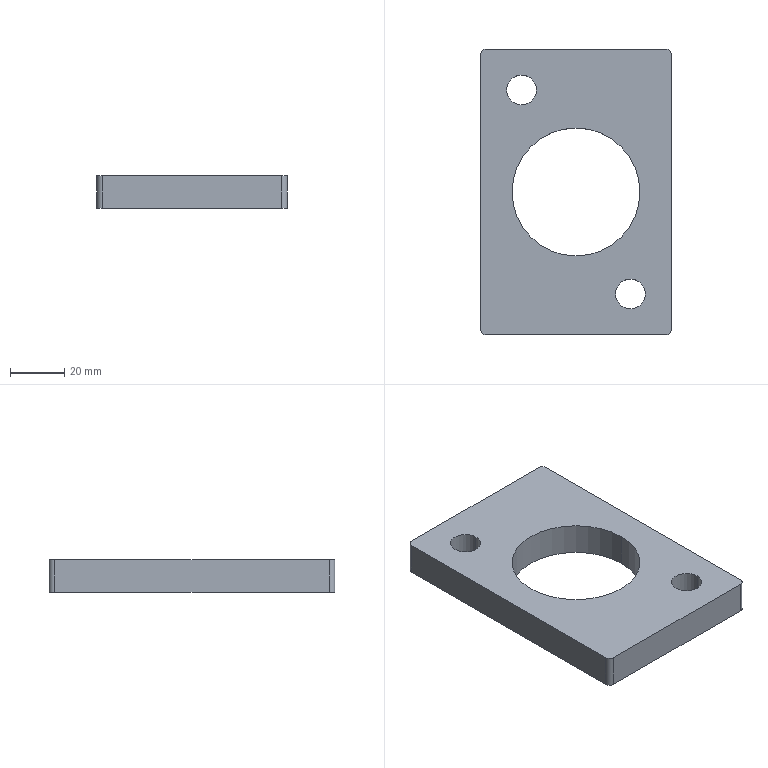Part | SolidWorks | features Extrusion 1 | 1 solid | 16 faces | box 70 x 105 x 12 mm | volume 65059 mm3 | cylinder 10 | plane 6 | commonest cylinder face diameters 4 x4 11 x4 47 x2
STEP:
#1=CARTESIAN_POINT('',(14.5,-37.5,12.));
#2=VERTEX_POINT('',#1);
#3=CARTESIAN_POINT('',(25.5,-37.5,12.));
#4=VERTEX_POINT('',#3);
#5=CARTESIAN_POINT('',(20.,-37.5,12.));
#6=DIRECTION('',(0.,0.,1.));
#7=DIRECTION('',(1.,0.,0.));
#8=AXIS2_PLACEMENT_3D('',#5,#6,#7);
#9=CIRCLE('',#8,5.5);
#10=EDGE_CURVE('',#2,#4,#9,.T.);
#11=ORIENTED_EDGE('',*,*,#10,.T.);
#12=CARTESIAN_POINT('',(25.5,-37.5,0.));
#13=VERTEX_POINT('',#12);
#14=CARTESIAN_POINT('',(25.5,-37.5,12.));
#15=DIRECTION('',(0.,0.,-1.));
#16=VECTOR('',#15,1000.);
#17=LINE('',#14,#16);
#18=EDGE_CURVE('',#4,#13,#17,.T.);
#19=ORIENTED_EDGE('',*,*,#18,.T.);
#20=CARTESIAN_POINT('',(14.5,-37.5,0.));
#21=VERTEX_POINT('',#20);
#22=CARTESIAN_POINT('',(20.,-37.5,0.));
#23=DIRECTION('',(0.,0.,1.));
#24=DIRECTION('',(1.,0.,0.));
#25=AXIS2_PLACEMENT_3D('',#22,#23,#24);
#26=CIRCLE('',#25,5.5);
#27=EDGE_CURVE('',#21,#13,#26,.T.);
#28=ORIENTED_EDGE('',*,*,#27,.F.);
#29=CARTESIAN_POINT('',(14.5,-37.5,12.));
#30=DIRECTION('',(0.,0.,-1.));
#31=VECTOR('',#30,1000.);
#32=LINE('',#29,#31);
#33=EDGE_CURVE('',#2,#21,#32,.T.);
#34=ORIENTED_EDGE('',*,*,#33,.F.);
#35=EDGE_LOOP('',(#11,#19,#28,#34));
#36=FACE_OUTER_BOUND('',#35,.T.);
#37=CARTESIAN_POINT('',(20.,-37.5,12.));
#38=DIRECTION('',(0.,0.,-1.));
#39=DIRECTION('',(-1.,0.,0.));
#40=AXIS2_PLACEMENT_3D('',#37,#38,#39);
#41=CYLINDRICAL_SURFACE('',#40,5.5);
#42=ADVANCED_FACE('',(#36),#41,.F.);
#43=CARTESIAN_POINT('',(-25.5,37.5,12.));
#44=VERTEX_POINT('',#43);
#45=CARTESIAN_POINT('',(-14.5,37.5,12.));
#46=VERTEX_POINT('',#45);
#47=CARTESIAN_POINT('',(-20.,37.5,12.));
#48=DIRECTION('',(0.,0.,1.));
#49=DIRECTION('',(1.,0.,0.));
#50=AXIS2_PLACEMENT_3D('',#47,#48,#49);
#51=CIRCLE('',#50,5.5);
#52=EDGE_CURVE('',#44,#46,#51,.T.);
#53=ORIENTED_EDGE('',*,*,#52,.T.);
#54=CARTESIAN_POINT('',(-14.5,37.5,0.));
#55=VERTEX_POINT('',#54);
#56=CARTESIAN_POINT('',(-14.5,37.5,12.));
#57=DIRECTION('',(0.,0.,-1.));
#58=VECTOR('',#57,1000.);
#59=LINE('',#56,#58);
#60=EDGE_CURVE('',#46,#55,#59,.T.);
#61=ORIENTED_EDGE('',*,*,#60,.T.);
#62=CARTESIAN_POINT('',(-25.5,37.5,0.));
#63=VERTEX_POINT('',#62);
#64=CARTESIAN_POINT('',(-20.,37.5,0.));
#65=DIRECTION('',(0.,0.,1.));
#66=DIRECTION('',(1.,0.,0.));
#67=AXIS2_PLACEMENT_3D('',#64,#65,#66);
#68=CIRCLE('',#67,5.5);
#69=EDGE_CURVE('',#63,#55,#68,.T.);
#70=ORIENTED_EDGE('',*,*,#69,.F.);
#71=CARTESIAN_POINT('',(-25.5,37.5,12.));
#72=DIRECTION('',(0.,0.,-1.));
#73=VECTOR('',#72,1000.);
#74=LINE('',#71,#73);
#75=EDGE_CURVE('',#44,#63,#74,.T.);
#76=ORIENTED_EDGE('',*,*,#75,.F.);
#77=EDGE_LOOP('',(#53,#61,#70,#76));
#78=FACE_OUTER_BOUND('',#77,.T.);
#79=CARTESIAN_POINT('',(-20.,37.5,12.));
#80=DIRECTION('',(0.,0.,-1.));
#81=DIRECTION('',(-1.,0.,0.));
#82=AXIS2_PLACEMENT_3D('',#79,#80,#81);
#83=CYLINDRICAL_SURFACE('',#82,5.5);
#84=ADVANCED_FACE('',(#78),#83,.F.);
#85=CARTESIAN_POINT('',(-23.5,0.,12.));
#86=VERTEX_POINT('',#85);
#87=CARTESIAN_POINT('',(23.5,0.,12.));
#88=VERTEX_POINT('',#87);
#89=CARTESIAN_POINT('',(0.,0.,12.));
#90=DIRECTION('',(0.,0.,1.));
#91=DIRECTION('',(1.,0.,0.));
#92=AXIS2_PLACEMENT_3D('',#89,#90,#91);
#93=CIRCLE('',#92,23.5);
#94=EDGE_CURVE('',#86,#88,#93,.T.);
#95=ORIENTED_EDGE('',*,*,#94,.T.);
#96=CARTESIAN_POINT('',(23.5,0.,0.));
#97=VERTEX_POINT('',#96);
#98=CARTESIAN_POINT('',(23.5,0.,12.));
#99=DIRECTION('',(0.,0.,-1.));
#100=VECTOR('',#99,1000.);
#101=LINE('',#98,#100);
#102=EDGE_CURVE('',#88,#97,#101,.T.);
#103=ORIENTED_EDGE('',*,*,#102,.T.);
#104=CARTESIAN_POINT('',(-23.5,0.,0.));
#105=VERTEX_POINT('',#104);
#106=CARTESIAN_POINT('',(0.,0.,0.));
#107=DIRECTION('',(0.,0.,1.));
#108=DIRECTION('',(1.,0.,0.));
#109=AXIS2_PLACEMENT_3D('',#106,#107,#108);
#110=CIRCLE('',#109,23.5);
#111=EDGE_CURVE('',#105,#97,#110,.T.);
#112=ORIENTED_EDGE('',*,*,#111,.F.);
#113=CARTESIAN_POINT('',(-23.5,0.,12.));
#114=DIRECTION('',(0.,0.,-1.));
#115=VECTOR('',#114,1000.);
#116=LINE('',#113,#115);
#117=EDGE_CURVE('',#86,#105,#116,.T.);
#118=ORIENTED_EDGE('',*,*,#117,.F.);
#119=EDGE_LOOP('',(#95,#103,#112,#118));
#120=FACE_OUTER_BOUND('',#119,.T.);
#121=CARTESIAN_POINT('',(0.,0.,12.));
#122=DIRECTION('',(0.,0.,-1.));
#123=DIRECTION('',(-1.,0.,0.));
#124=AXIS2_PLACEMENT_3D('',#121,#122,#123);
#125=CYLINDRICAL_SURFACE('',#124,23.5);
#126=ADVANCED_FACE('',(#120),#125,.F.);
#127=ORIENTED_EDGE('',*,*,#52,.F.);
#128=CARTESIAN_POINT('',(-20.,37.5,12.));
#129=DIRECTION('',(0.,0.,1.));
#130=DIRECTION('',(1.,0.,0.));
#131=AXIS2_PLACEMENT_3D('',#128,#129,#130);
#132=CIRCLE('',#131,5.5);
#133=EDGE_CURVE('',#46,#44,#132,.T.);
#134=ORIENTED_EDGE('',*,*,#133,.F.);
#135=EDGE_LOOP('',(#127,#134));
#136=FACE_BOUND('',#135,.T.);
#137=CARTESIAN_POINT('',(-33.,52.5,12.));
#138=VERTEX_POINT('',#137);
#139=CARTESIAN_POINT('',(-35.,50.5,12.));
#140=VERTEX_POINT('',#139);
#141=CARTESIAN_POINT('',(-33.,50.5,12.));
#142=DIRECTION('',(0.,0.,1.));
#143=DIRECTION('',(1.,0.,0.));
#144=AXIS2_PLACEMENT_3D('',#141,#142,#143);
#145=CIRCLE('',#144,2.);
#146=EDGE_CURVE('',#138,#140,#145,.T.);
#147=ORIENTED_EDGE('',*,*,#146,.T.);
#148=CARTESIAN_POINT('',(-35.,-50.5,12.));
#149=VERTEX_POINT('',#148);
#150=CARTESIAN_POINT('',(-35.,50.5,12.));
#151=DIRECTION('',(0.,-1.,0.));
#152=VECTOR('',#151,1000.);
#153=LINE('',#150,#152);
#154=EDGE_CURVE('',#140,#149,#153,.T.);
#155=ORIENTED_EDGE('',*,*,#154,.T.);
#156=CARTESIAN_POINT('',(-33.,-52.5,12.));
#157=VERTEX_POINT('',#156);
#158=CARTESIAN_POINT('',(-33.,-50.5,12.));
#159=DIRECTION('',(0.,0.,1.));
#160=DIRECTION('',(1.,0.,0.));
#161=AXIS2_PLACEMENT_3D('',#158,#159,#160);
#162=CIRCLE('',#161,2.);
#163=EDGE_CURVE('',#149,#157,#162,.T.);
#164=ORIENTED_EDGE('',*,*,#163,.T.);
#165=CARTESIAN_POINT('',(33.,-52.5,12.));
#166=VERTEX_POINT('',#165);
#167=CARTESIAN_POINT('',(-33.,-52.5,12.));
#168=DIRECTION('',(1.,0.,0.));
#169=VECTOR('',#168,1000.);
#170=LINE('',#167,#169);
#171=EDGE_CURVE('',#157,#166,#170,.T.);
#172=ORIENTED_EDGE('',*,*,#171,.T.);
#173=CARTESIAN_POINT('',(35.,-50.5,12.));
#174=VERTEX_POINT('',#173);
#175=CARTESIAN_POINT('',(33.,-50.5,12.));
#176=DIRECTION('',(0.,0.,1.));
#177=DIRECTION('',(1.,0.,0.));
#178=AXIS2_PLACEMENT_3D('',#175,#176,#177);
#179=CIRCLE('',#178,2.);
#180=EDGE_CURVE('',#166,#174,#179,.T.);
#181=ORIENTED_EDGE('',*,*,#180,.T.);
#182=CARTESIAN_POINT('',(35.,50.5,12.));
#183=VERTEX_POINT('',#182);
#184=CARTESIAN_POINT('',(35.,50.5,12.));
#185=DIRECTION('',(0.,1.,0.));
#186=VECTOR('',#185,1000.);
#187=LINE('',#184,#186);
#188=EDGE_CURVE('',#174,#183,#187,.T.);
#189=ORIENTED_EDGE('',*,*,#188,.T.);
#190=CARTESIAN_POINT('',(33.,52.5,12.));
#191=VERTEX_POINT('',#190);
#192=CARTESIAN_POINT('',(33.,50.5,12.));
#193=DIRECTION('',(0.,0.,1.));
#194=DIRECTION('',(-1.,0.,0.));
#195=AXIS2_PLACEMENT_3D('',#192,#193,#194);
#196=CIRCLE('',#195,2.);
#197=EDGE_CURVE('',#183,#191,#196,.T.);
#198=ORIENTED_EDGE('',*,*,#197,.T.);
#199=CARTESIAN_POINT('',(-33.,52.5,12.));
#200=DIRECTION('',(-1.,0.,0.));
#201=VECTOR('',#200,1000.);
#202=LINE('',#199,#201);
#203=EDGE_CURVE('',#191,#138,#202,.T.);
#204=ORIENTED_EDGE('',*,*,#203,.T.);
#205=EDGE_LOOP('',(#147,#155,#164,#172,#181,#189,#198,#204));
#206=FACE_OUTER_BOUND('',#205,.T.);
#207=ORIENTED_EDGE('',*,*,#94,.F.);
#208=CARTESIAN_POINT('',(0.,0.,12.));
#209=DIRECTION('',(0.,0.,1.));
#210=DIRECTION('',(1.,0.,0.));
#211=AXIS2_PLACEMENT_3D('',#208,#209,#210);
#212=CIRCLE('',#211,23.5);
#213=EDGE_CURVE('',#88,#86,#212,.T.);
#214=ORIENTED_EDGE('',*,*,#213,.F.);
#215=EDGE_LOOP('',(#207,#214));
#216=FACE_BOUND('',#215,.T.);
#217=ORIENTED_EDGE('',*,*,#10,.F.);
#218=CARTESIAN_POINT('',(20.,-37.5,12.));
#219=DIRECTION('',(0.,0.,1.));
#220=DIRECTION('',(1.,0.,0.));
#221=AXIS2_PLACEMENT_3D('',#218,#219,#220);
#222=CIRCLE('',#221,5.5);
#223=EDGE_CURVE('',#4,#2,#222,.T.);
#224=ORIENTED_EDGE('',*,*,#223,.F.);
#225=EDGE_LOOP('',(#217,#224));
#226=FACE_BOUND('',#225,.T.);
#227=CARTESIAN_POINT('',(-33.,50.5,12.));
#228=DIRECTION('',(0.,0.,1.));
#229=DIRECTION('',(1.,0.,0.));
#230=AXIS2_PLACEMENT_3D('',#227,#228,#229);
#231=PLANE('',#230);
#232=ADVANCED_FACE('',(#136,#206,#216,#226),#231,.T.);
#233=CARTESIAN_POINT('',(-33.,52.5,0.));
#234=VERTEX_POINT('',#233);
#235=CARTESIAN_POINT('',(-35.,50.5,0.));
#236=VERTEX_POINT('',#235);
#237=CARTESIAN_POINT('',(-33.,50.5,0.));
#238=DIRECTION('',(0.,0.,1.));
#239=DIRECTION('',(1.,0.,0.));
#240=AXIS2_PLACEMENT_3D('',#237,#238,#239);
#241=CIRCLE('',#240,2.);
#242=EDGE_CURVE('',#234,#236,#241,.T.);
#243=ORIENTED_EDGE('',*,*,#242,.F.);
#244=CARTESIAN_POINT('',(33.,52.5,0.));
#245=VERTEX_POINT('',#244);
#246=CARTESIAN_POINT('',(-33.,52.5,0.));
#247=DIRECTION('',(-1.,0.,0.));
#248=VECTOR('',#247,1000.);
#249=LINE('',#246,#248);
#250=EDGE_CURVE('',#245,#234,#249,.T.);
#251=ORIENTED_EDGE('',*,*,#250,.F.);
#252=CARTESIAN_POINT('',(35.,50.5,0.));
#253=VERTEX_POINT('',#252);
#254=CARTESIAN_POINT('',(33.,50.5,0.));
#255=DIRECTION('',(0.,0.,1.));
#256=DIRECTION('',(-1.,0.,0.));
#257=AXIS2_PLACEMENT_3D('',#254,#255,#256);
#258=CIRCLE('',#257,2.);
#259=EDGE_CURVE('',#253,#245,#258,.T.);
#260=ORIENTED_EDGE('',*,*,#259,.F.);
#261=CARTESIAN_POINT('',(35.,-50.5,0.));
#262=VERTEX_POINT('',#261);
#263=CARTESIAN_POINT('',(35.,50.5,0.));
#264=DIRECTION('',(0.,1.,0.));
#265=VECTOR('',#264,1000.);
#266=LINE('',#263,#265);
#267=EDGE_CURVE('',#262,#253,#266,.T.);
#268=ORIENTED_EDGE('',*,*,#267,.F.);
#269=CARTESIAN_POINT('',(33.,-52.5,0.));
#270=VERTEX_POINT('',#269);
#271=CARTESIAN_POINT('',(33.,-50.5,0.));
#272=DIRECTION('',(0.,0.,1.));
#273=DIRECTION('',(1.,0.,0.));
#274=AXIS2_PLACEMENT_3D('',#271,#272,#273);
#275=CIRCLE('',#274,2.);
#276=EDGE_CURVE('',#270,#262,#275,.T.);
#277=ORIENTED_EDGE('',*,*,#276,.F.);
#278=CARTESIAN_POINT('',(-33.,-52.5,0.));
#279=VERTEX_POINT('',#278);
#280=CARTESIAN_POINT('',(-33.,-52.5,0.));
#281=DIRECTION('',(1.,0.,0.));
#282=VECTOR('',#281,1000.);
#283=LINE('',#280,#282);
#284=EDGE_CURVE('',#279,#270,#283,.T.);
#285=ORIENTED_EDGE('',*,*,#284,.F.);
#286=CARTESIAN_POINT('',(-35.,-50.5,0.));
#287=VERTEX_POINT('',#286);
#288=CARTESIAN_POINT('',(-33.,-50.5,0.));
#289=DIRECTION('',(0.,0.,1.));
#290=DIRECTION('',(1.,0.,0.));
#291=AXIS2_PLACEMENT_3D('',#288,#289,#290);
#292=CIRCLE('',#291,2.);
#293=EDGE_CURVE('',#287,#279,#292,.T.);
#294=ORIENTED_EDGE('',*,*,#293,.F.);
#295=CARTESIAN_POINT('',(-35.,50.5,0.));
#296=DIRECTION('',(0.,-1.,0.));
#297=VECTOR('',#296,1000.);
#298=LINE('',#295,#297);
#299=EDGE_CURVE('',#236,#287,#298,.T.);
#300=ORIENTED_EDGE('',*,*,#299,.F.);
#301=EDGE_LOOP('',(#243,#251,#260,#268,#277,#285,#294,#300));
#302=FACE_OUTER_BOUND('',#301,.T.);
#303=ORIENTED_EDGE('',*,*,#111,.T.);
#304=CARTESIAN_POINT('',(0.,0.,0.));
#305=DIRECTION('',(0.,0.,1.));
#306=DIRECTION('',(1.,0.,0.));
#307=AXIS2_PLACEMENT_3D('',#304,#305,#306);
#308=CIRCLE('',#307,23.5);
#309=EDGE_CURVE('',#97,#105,#308,.T.);
#310=ORIENTED_EDGE('',*,*,#309,.T.);
#311=EDGE_LOOP('',(#303,#310));
#312=FACE_BOUND('',#311,.T.);
#313=ORIENTED_EDGE('',*,*,#69,.T.);
#314=CARTESIAN_POINT('',(-20.,37.5,0.));
#315=DIRECTION('',(0.,0.,1.));
#316=DIRECTION('',(1.,0.,0.));
#317=AXIS2_PLACEMENT_3D('',#314,#315,#316);
#318=CIRCLE('',#317,5.5);
#319=EDGE_CURVE('',#55,#63,#318,.T.);
#320=ORIENTED_EDGE('',*,*,#319,.T.);
#321=EDGE_LOOP('',(#313,#320));
#322=FACE_BOUND('',#321,.T.);
#323=ORIENTED_EDGE('',*,*,#27,.T.);
#324=CARTESIAN_POINT('',(20.,-37.5,0.));
#325=DIRECTION('',(0.,0.,1.));
#326=DIRECTION('',(1.,0.,0.));
#327=AXIS2_PLACEMENT_3D('',#324,#325,#326);
#328=CIRCLE('',#327,5.5);
#329=EDGE_CURVE('',#13,#21,#328,.T.);
#330=ORIENTED_EDGE('',*,*,#329,.T.);
#331=EDGE_LOOP('',(#323,#330));
#332=FACE_BOUND('',#331,.T.);
#333=CARTESIAN_POINT('',(-33.,50.5,0.));
#334=DIRECTION('',(0.,0.,1.));
#335=DIRECTION('',(1.,0.,0.));
#336=AXIS2_PLACEMENT_3D('',#333,#334,#335);
#337=PLANE('',#336);
#338=ADVANCED_FACE('',(#302,#312,#322,#332),#337,.F.);
#339=ORIENTED_EDGE('',*,*,#242,.T.);
#340=CARTESIAN_POINT('',(-35.,50.5,12.));
#341=DIRECTION('',(0.,0.,-1.));
#342=VECTOR('',#341,1000.);
#343=LINE('',#340,#342);
#344=EDGE_CURVE('',#140,#236,#343,.T.);
#345=ORIENTED_EDGE('',*,*,#344,.F.);
#346=ORIENTED_EDGE('',*,*,#146,.F.);
#347=CARTESIAN_POINT('',(-33.,52.5,12.));
#348=DIRECTION('',(0.,0.,-1.));
#349=VECTOR('',#348,1000.);
#350=LINE('',#347,#349);
#351=EDGE_CURVE('',#138,#234,#350,.T.);
#352=ORIENTED_EDGE('',*,*,#351,.T.);
#353=EDGE_LOOP('',(#339,#345,#346,#352));
#354=FACE_OUTER_BOUND('',#353,.T.);
#355=CARTESIAN_POINT('',(-33.,50.5,12.));
#356=DIRECTION('',(0.,0.,-1.));
#357=DIRECTION('',(-1.,0.,0.));
#358=AXIS2_PLACEMENT_3D('',#355,#356,#357);
#359=CYLINDRICAL_SURFACE('',#358,2.);
#360=ADVANCED_FACE('',(#354),#359,.T.);
#361=ORIENTED_EDGE('',*,*,#299,.T.);
#362=CARTESIAN_POINT('',(-35.,-50.5,12.));
#363=DIRECTION('',(0.,0.,-1.));
#364=VECTOR('',#363,1000.);
#365=LINE('',#362,#364);
#366=EDGE_CURVE('',#149,#287,#365,.T.);
#367=ORIENTED_EDGE('',*,*,#366,.F.);
#368=ORIENTED_EDGE('',*,*,#154,.F.);
#369=ORIENTED_EDGE('',*,*,#344,.T.);
#370=EDGE_LOOP('',(#361,#367,#368,#369));
#371=FACE_OUTER_BOUND('',#370,.T.);
#372=CARTESIAN_POINT('',(-35.,50.5,12.));
#373=DIRECTION('',(1.,0.,0.));
#374=DIRECTION('',(0.,1.,0.));
#375=AXIS2_PLACEMENT_3D('',#372,#373,#374);
#376=PLANE('',#375);
#377=ADVANCED_FACE('',(#371),#376,.F.);
#378=ORIENTED_EDGE('',*,*,#293,.T.);
#379=CARTESIAN_POINT('',(-33.,-52.5,12.));
#380=DIRECTION('',(0.,0.,-1.));
#381=VECTOR('',#380,1000.);
#382=LINE('',#379,#381);
#383=EDGE_CURVE('',#157,#279,#382,.T.);
#384=ORIENTED_EDGE('',*,*,#383,.F.);
#385=ORIENTED_EDGE('',*,*,#163,.F.);
#386=ORIENTED_EDGE('',*,*,#366,.T.);
#387=EDGE_LOOP('',(#378,#384,#385,#386));
#388=FACE_OUTER_BOUND('',#387,.T.);
#389=CARTESIAN_POINT('',(-33.,-50.5,12.));
#390=DIRECTION('',(0.,0.,-1.));
#391=DIRECTION('',(-1.,0.,0.));
#392=AXIS2_PLACEMENT_3D('',#389,#390,#391);
#393=CYLINDRICAL_SURFACE('',#392,2.);
#394=ADVANCED_FACE('',(#388),#393,.T.);
#395=ORIENTED_EDGE('',*,*,#284,.T.);
#396=CARTESIAN_POINT('',(33.,-52.5,12.));
#397=DIRECTION('',(0.,0.,-1.));
#398=VECTOR('',#397,1000.);
#399=LINE('',#396,#398);
#400=EDGE_CURVE('',#166,#270,#399,.T.);
#401=ORIENTED_EDGE('',*,*,#400,.F.);
#402=ORIENTED_EDGE('',*,*,#171,.F.);
#403=ORIENTED_EDGE('',*,*,#383,.T.);
#404=EDGE_LOOP('',(#395,#401,#402,#403));
#405=FACE_OUTER_BOUND('',#404,.T.);
#406=CARTESIAN_POINT('',(-33.,-52.5,12.));
#407=DIRECTION('',(0.,1.,0.));
#408=DIRECTION('',(0.,0.,1.));
#409=AXIS2_PLACEMENT_3D('',#406,#407,#408);
#410=PLANE('',#409);
#411=ADVANCED_FACE('',(#405),#410,.F.);
#412=ORIENTED_EDGE('',*,*,#276,.T.);
#413=CARTESIAN_POINT('',(35.,-50.5,12.));
#414=DIRECTION('',(0.,0.,-1.));
#415=VECTOR('',#414,1000.);
#416=LINE('',#413,#415);
#417=EDGE_CURVE('',#174,#262,#416,.T.);
#418=ORIENTED_EDGE('',*,*,#417,.F.);
#419=ORIENTED_EDGE('',*,*,#180,.F.);
#420=ORIENTED_EDGE('',*,*,#400,.T.);
#421=EDGE_LOOP('',(#412,#418,#419,#420));
#422=FACE_OUTER_BOUND('',#421,.T.);
#423=CARTESIAN_POINT('',(33.,-50.5,12.));
#424=DIRECTION('',(0.,0.,-1.));
#425=DIRECTION('',(-1.,0.,0.));
#426=AXIS2_PLACEMENT_3D('',#423,#424,#425);
#427=CYLINDRICAL_SURFACE('',#426,2.);
#428=ADVANCED_FACE('',(#422),#427,.T.);
#429=ORIENTED_EDGE('',*,*,#267,.T.);
#430=CARTESIAN_POINT('',(35.,50.5,12.));
#431=DIRECTION('',(0.,0.,-1.));
#432=VECTOR('',#431,1000.);
#433=LINE('',#430,#432);
#434=EDGE_CURVE('',#183,#253,#433,.T.);
#435=ORIENTED_EDGE('',*,*,#434,.F.);
#436=ORIENTED_EDGE('',*,*,#188,.F.);
#437=ORIENTED_EDGE('',*,*,#417,.T.);
#438=EDGE_LOOP('',(#429,#435,#436,#437));
#439=FACE_OUTER_BOUND('',#438,.T.);
#440=CARTESIAN_POINT('',(35.,50.5,12.));
#441=DIRECTION('',(-1.,0.,0.));
#442=DIRECTION('',(0.,-1.,0.));
#443=AXIS2_PLACEMENT_3D('',#440,#441,#442);
#444=PLANE('',#443);
#445=ADVANCED_FACE('',(#439),#444,.F.);
#446=ORIENTED_EDGE('',*,*,#259,.T.);
#447=CARTESIAN_POINT('',(33.,52.5,12.));
#448=DIRECTION('',(0.,0.,-1.));
#449=VECTOR('',#448,1000.);
#450=LINE('',#447,#449);
#451=EDGE_CURVE('',#191,#245,#450,.T.);
#452=ORIENTED_EDGE('',*,*,#451,.F.);
#453=ORIENTED_EDGE('',*,*,#197,.F.);
#454=ORIENTED_EDGE('',*,*,#434,.T.);
#455=EDGE_LOOP('',(#446,#452,#453,#454));
#456=FACE_OUTER_BOUND('',#455,.T.);
#457=CARTESIAN_POINT('',(33.,50.5,12.));
#458=DIRECTION('',(0.,0.,-1.));
#459=DIRECTION('',(-1.,0.,0.));
#460=AXIS2_PLACEMENT_3D('',#457,#458,#459);
#461=CYLINDRICAL_SURFACE('',#460,2.);
#462=ADVANCED_FACE('',(#456),#461,.T.);
#463=ORIENTED_EDGE('',*,*,#250,.T.);
#464=ORIENTED_EDGE('',*,*,#351,.F.);
#465=ORIENTED_EDGE('',*,*,#203,.F.);
#466=ORIENTED_EDGE('',*,*,#451,.T.);
#467=EDGE_LOOP('',(#463,#464,#465,#466));
#468=FACE_OUTER_BOUND('',#467,.T.);
#469=CARTESIAN_POINT('',(-33.,52.5,12.));
#470=DIRECTION('',(0.,-1.,0.));
#471=DIRECTION('',(0.,0.,-1.));
#472=AXIS2_PLACEMENT_3D('',#469,#470,#471);
#473=PLANE('',#472);
#474=ADVANCED_FACE('',(#468),#473,.F.);
#475=ORIENTED_EDGE('',*,*,#102,.F.);
#476=ORIENTED_EDGE('',*,*,#213,.T.);
#477=ORIENTED_EDGE('',*,*,#117,.T.);
#478=ORIENTED_EDGE('',*,*,#309,.F.);
#479=EDGE_LOOP('',(#475,#476,#477,#478));
#480=FACE_OUTER_BOUND('',#479,.T.);
#481=CARTESIAN_POINT('',(0.,0.,12.));
#482=DIRECTION('',(0.,0.,-1.));
#483=DIRECTION('',(-1.,0.,0.));
#484=AXIS2_PLACEMENT_3D('',#481,#482,#483);
#485=CYLINDRICAL_SURFACE('',#484,23.5);
#486=ADVANCED_FACE('',(#480),#485,.F.);
#487=ORIENTED_EDGE('',*,*,#60,.F.);
#488=ORIENTED_EDGE('',*,*,#133,.T.);
#489=ORIENTED_EDGE('',*,*,#75,.T.);
#490=ORIENTED_EDGE('',*,*,#319,.F.);
#491=EDGE_LOOP('',(#487,#488,#489,#490));
#492=FACE_OUTER_BOUND('',#491,.T.);
#493=CARTESIAN_POINT('',(-20.,37.5,12.));
#494=DIRECTION('',(0.,0.,-1.));
#495=DIRECTION('',(-1.,0.,0.));
#496=AXIS2_PLACEMENT_3D('',#493,#494,#495);
#497=CYLINDRICAL_SURFACE('',#496,5.5);
#498=ADVANCED_FACE('',(#492),#497,.F.);
#499=ORIENTED_EDGE('',*,*,#18,.F.);
#500=ORIENTED_EDGE('',*,*,#223,.T.);
#501=ORIENTED_EDGE('',*,*,#33,.T.);
#502=ORIENTED_EDGE('',*,*,#329,.F.);
#503=EDGE_LOOP('',(#499,#500,#501,#502));
#504=FACE_OUTER_BOUND('',#503,.T.);
#505=CARTESIAN_POINT('',(20.,-37.5,12.));
#506=DIRECTION('',(0.,0.,-1.));
#507=DIRECTION('',(-1.,0.,0.));
#508=AXIS2_PLACEMENT_3D('',#505,#506,#507);
#509=CYLINDRICAL_SURFACE('',#508,5.5);
#510=ADVANCED_FACE('',(#504),#509,.F.);
#511=CLOSED_SHELL('',(#42,#84,#126,#232,#338,#360,#377,#394,#411,#428,#445,#462,#474,#486,#498,#510));
#512=MANIFOLD_SOLID_BREP('',#511);
#513=CARTESIAN_POINT('',(0.,0.,0.));
#514=DIRECTION('',(0.,0.,1.));
#515=DIRECTION('',(1.,0.,0.));
#516=AXIS2_PLACEMENT_3D('',#513,#514,#515);
#517=(LENGTH_UNIT()NAMED_UNIT(*)SI_UNIT(.MILLI.,.METRE.));
#518=UNCERTAINTY_MEASURE_WITH_UNIT(LENGTH_MEASURE(0.00001),#517,'','');
#519=(NAMED_UNIT(*)PLANE_ANGLE_UNIT()SI_UNIT($,.RADIAN.));
#520=(NAMED_UNIT(*)SI_UNIT($,.STERADIAN.)SOLID_ANGLE_UNIT());
#521=(GEOMETRIC_REPRESENTATION_CONTEXT(3)GLOBAL_UNCERTAINTY_ASSIGNED_CONTEXT((#518))GLOBAL_UNIT_ASSIGNED_CONTEXT((#517,#519,#520))REPRESENTATION_CONTEXT('',''));
#522=ADVANCED_BREP_SHAPE_REPRESENTATION('',(#512,#516),#521);